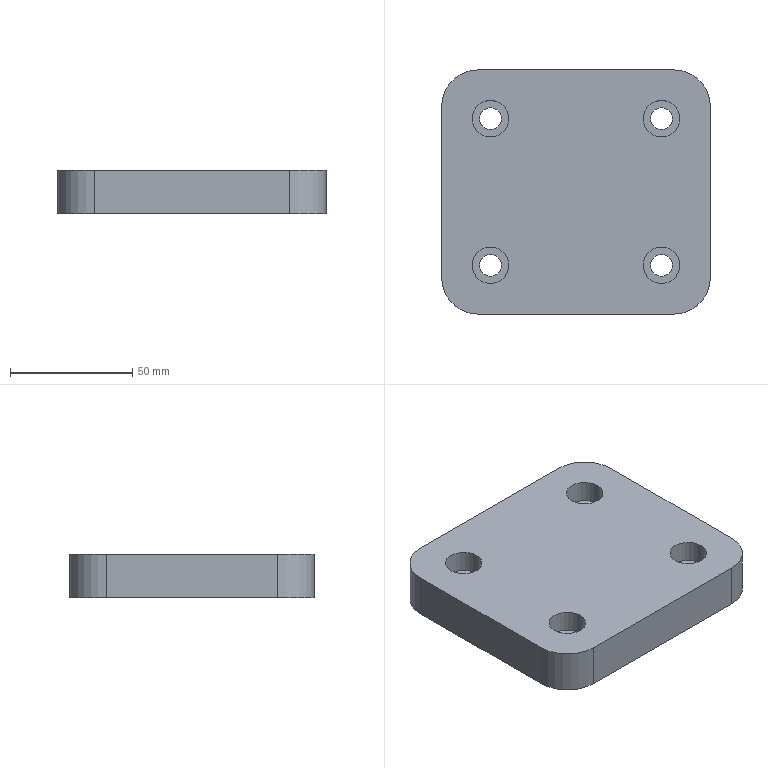Part | STEP file | solid 52 | 1 solid | 22 faces | box 110 x 100 x 18 mm | volume 185872 mm3 | cylinder 12 | plane 10 | commonest cylinder face diameters 9 x4 15 x4 30 x4